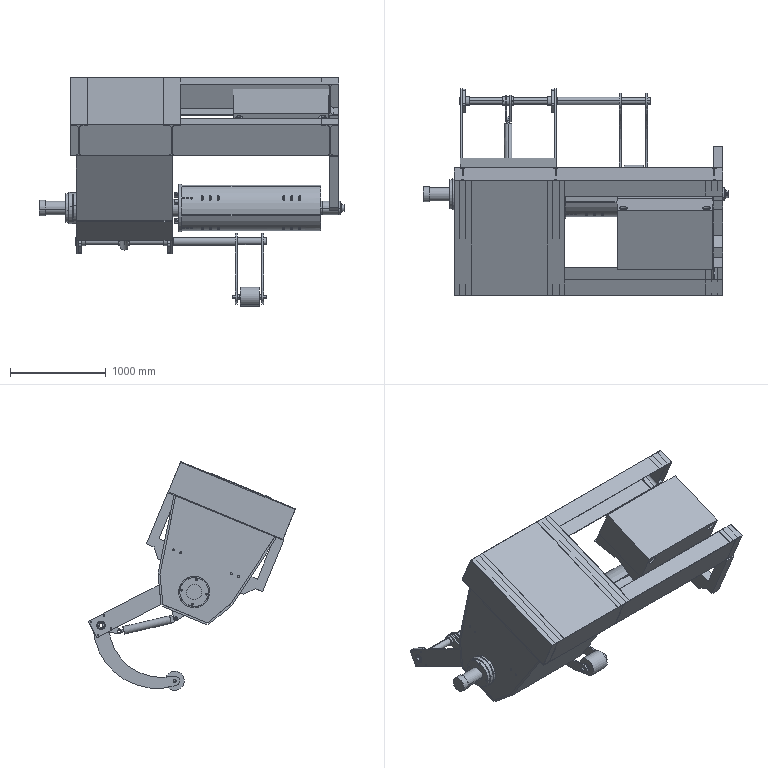Part | SolidWorks | 157 solids | 4264 faces | volume 464591008 mm3 | cylinder 1974 | plane 1264 | torus 318 | spline 303 | sphere 300 | cone 105 | commonest cylinder face diameters 12.5 x280 50 x150 22.807 x136 41.467 x136 22 x104 170 x97